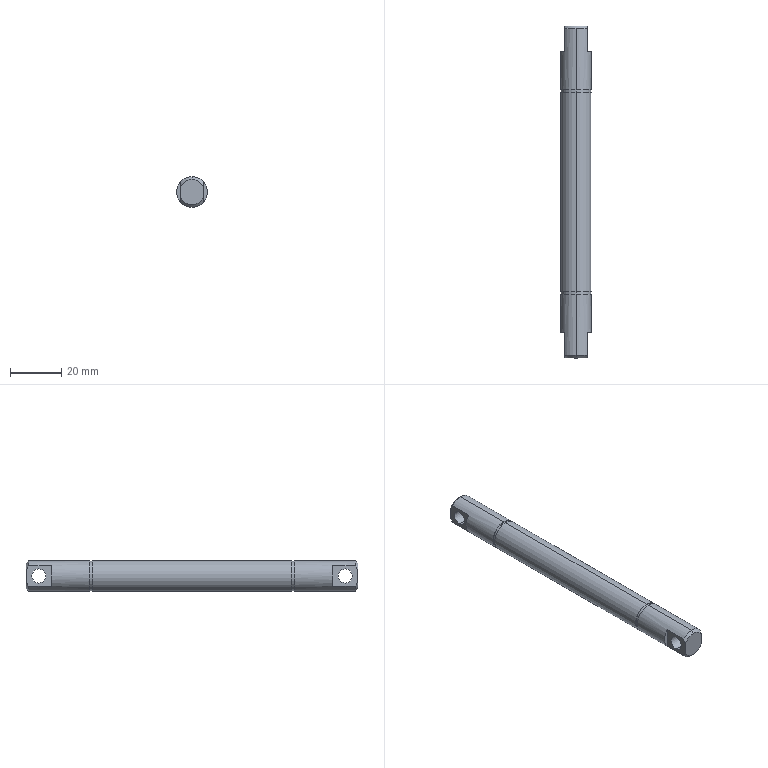Part | SolidWorks | features ICE 3, MirrorPattern 3, Chamfer 1, Extrusion 1 | 1 solid | 34 faces | box 12 x 130 x 12 mm | volume 13909 mm3 | cylinder 14 | plane 14 | cone 6 | commonest cylinder face diameters 12 x6 5.5 x4 11.5 x4
STEP:
#1=CARTESIAN_POINT('',(0.,25.,6.));
#2=VERTEX_POINT('',#1);
#3=CARTESIAN_POINT('',(0.,25.,-6.));
#4=VERTEX_POINT('',#3);
#5=CARTESIAN_POINT('',(0.,25.,0.));
#6=DIRECTION('',(0.,1.,0.));
#7=DIRECTION('',(0.,0.,1.));
#8=AXIS2_PLACEMENT_3D('',#5,#6,#7);
#9=CIRCLE('',#8,6.);
#10=EDGE_CURVE('',#2,#4,#9,.T.);
#11=ORIENTED_EDGE('',*,*,#10,.F.);
#12=CARTESIAN_POINT('',(0.,1.,6.));
#13=VERTEX_POINT('',#12);
#14=CARTESIAN_POINT('',(0.,130.,6.));
#15=DIRECTION('',(0.,-1.,0.));
#16=VECTOR('',#15,1000.);
#17=LINE('',#14,#16);
#18=EDGE_CURVE('',#2,#13,#17,.T.);
#19=ORIENTED_EDGE('',*,*,#18,.T.);
#20=CARTESIAN_POINT('',(4.5,1.,3.969));
#21=VERTEX_POINT('',#20);
#22=CARTESIAN_POINT('',(0.,1.,0.));
#23=DIRECTION('',(0.,1.,0.));
#24=DIRECTION('',(0.,0.,1.));
#25=AXIS2_PLACEMENT_3D('',#22,#23,#24);
#26=CIRCLE('',#25,6.);
#27=EDGE_CURVE('',#13,#21,#26,.T.);
#28=ORIENTED_EDGE('',*,*,#27,.T.);
#29=CARTESIAN_POINT('',(4.5,10.,3.969));
#30=VERTEX_POINT('',#29);
#31=CARTESIAN_POINT('',(4.5,130.,3.969));
#32=DIRECTION('',(0.,1.,0.));
#33=VECTOR('',#32,1000.);
#34=LINE('',#31,#33);
#35=EDGE_CURVE('',#21,#30,#34,.T.);
#36=ORIENTED_EDGE('',*,*,#35,.T.);
#37=CARTESIAN_POINT('',(4.5,10.,-3.969));
#38=VERTEX_POINT('',#37);
#39=CARTESIAN_POINT('',(0.,10.,0.));
#40=DIRECTION('',(0.,1.,0.));
#41=DIRECTION('',(0.,0.,1.));
#42=AXIS2_PLACEMENT_3D('',#39,#40,#41);
#43=CIRCLE('',#42,6.);
#44=EDGE_CURVE('',#30,#38,#43,.T.);
#45=ORIENTED_EDGE('',*,*,#44,.T.);
#46=CARTESIAN_POINT('',(4.5,1.,-3.969));
#47=VERTEX_POINT('',#46);
#48=CARTESIAN_POINT('',(4.5,130.,-3.969));
#49=DIRECTION('',(0.,-1.,0.));
#50=VECTOR('',#49,1000.);
#51=LINE('',#48,#50);
#52=EDGE_CURVE('',#38,#47,#51,.T.);
#53=ORIENTED_EDGE('',*,*,#52,.T.);
#54=CARTESIAN_POINT('',(0.,1.,-6.));
#55=VERTEX_POINT('',#54);
#56=CARTESIAN_POINT('',(0.,1.,0.));
#57=DIRECTION('',(0.,1.,0.));
#58=DIRECTION('',(0.,0.,1.));
#59=AXIS2_PLACEMENT_3D('',#56,#57,#58);
#60=CIRCLE('',#59,6.);
#61=EDGE_CURVE('',#47,#55,#60,.T.);
#62=ORIENTED_EDGE('',*,*,#61,.T.);
#63=CARTESIAN_POINT('',(0.,130.,-6.));
#64=DIRECTION('',(0.,-1.,0.));
#65=VECTOR('',#64,1000.);
#66=LINE('',#63,#65);
#67=EDGE_CURVE('',#4,#55,#66,.T.);
#68=ORIENTED_EDGE('',*,*,#67,.F.);
#69=EDGE_LOOP('',(#11,#19,#28,#36,#45,#53,#62,#68));
#70=FACE_OUTER_BOUND('',#69,.T.);
#71=CARTESIAN_POINT('',(0.,130.,0.));
#72=DIRECTION('',(0.,-1.,0.));
#73=DIRECTION('',(0.,0.,-1.));
#74=AXIS2_PLACEMENT_3D('',#71,#72,#73);
#75=CYLINDRICAL_SURFACE('',#74,6.);
#76=ADVANCED_FACE('',(#70),#75,.T.);
#77=CARTESIAN_POINT('',(0.,0.,5.));
#78=VERTEX_POINT('',#77);
#79=CARTESIAN_POINT('',(-4.5,0.,2.179));
#80=VERTEX_POINT('',#79);
#81=CARTESIAN_POINT('',(0.,0.,0.));
#82=DIRECTION('',(0.,-1.,0.));
#83=DIRECTION('',(0.,0.,1.));
#84=AXIS2_PLACEMENT_3D('',#81,#82,#83);
#85=CIRCLE('',#84,5.);
#86=EDGE_CURVE('',#78,#80,#85,.T.);
#87=ORIENTED_EDGE('',*,*,#86,.F.);
#88=CARTESIAN_POINT('',(0.,1.,6.));
#89=DIRECTION('',(0.,0.7071,0.7071));
#90=VECTOR('',#89,1000.);
#91=LINE('',#88,#90);
#92=EDGE_CURVE('',#78,#13,#91,.T.);
#93=ORIENTED_EDGE('',*,*,#92,.T.);
#94=CARTESIAN_POINT('',(-4.5,1.,3.969));
#95=VERTEX_POINT('',#94);
#96=CARTESIAN_POINT('',(0.,1.,0.));
#97=DIRECTION('',(0.,1.,0.));
#98=DIRECTION('',(0.,0.,1.));
#99=AXIS2_PLACEMENT_3D('',#96,#97,#98);
#100=CIRCLE('',#99,6.);
#101=EDGE_CURVE('',#95,#13,#100,.T.);
#102=ORIENTED_EDGE('',*,*,#101,.F.);
#103=CARTESIAN_POINT('',(-4.5,0.,2.179));
#104=CARTESIAN_POINT('',(-4.5,0.2738,2.808));
#105=CARTESIAN_POINT('',(-4.5,0.6215,3.396));
#106=CARTESIAN_POINT('',(-4.5,1.,3.969));
#107=B_SPLINE_CURVE_WITH_KNOTS('',3,(#103,#104,#105,#106),.UNSPECIFIED.,.F.,.F.,(4,4),(0.006523,0.008562),.UNSPECIFIED.);
#108=EDGE_CURVE('',#80,#95,#107,.T.);
#109=ORIENTED_EDGE('',*,*,#108,.F.);
#110=EDGE_LOOP('',(#87,#93,#102,#109));
#111=FACE_OUTER_BOUND('',#110,.T.);
#112=CARTESIAN_POINT('',(0.,1.,0.));
#113=DIRECTION('',(0.,1.,0.));
#114=DIRECTION('',(0.,0.,1.));
#115=AXIS2_PLACEMENT_3D('',#112,#113,#114);
#116=CONICAL_SURFACE('',#115,6.,0.7854);
#117=ADVANCED_FACE('',(#111),#116,.T.);
#118=CARTESIAN_POINT('',(-4.5,5.,-2.75));
#119=VERTEX_POINT('',#118);
#120=CARTESIAN_POINT('',(-4.5,5.,2.75));
#121=VERTEX_POINT('',#120);
#122=CARTESIAN_POINT('',(-4.5,5.,0.));
#123=DIRECTION('',(-1.,0.,0.));
#124=DIRECTION('',(0.,0.,-1.));
#125=AXIS2_PLACEMENT_3D('',#122,#123,#124);
#126=CIRCLE('',#125,2.75);
#127=EDGE_CURVE('',#119,#121,#126,.T.);
#128=ORIENTED_EDGE('',*,*,#127,.T.);
#129=CARTESIAN_POINT('',(4.5,5.,2.75));
#130=VERTEX_POINT('',#129);
#131=CARTESIAN_POINT('',(-6.,5.,2.75));
#132=DIRECTION('',(1.,0.,0.));
#133=VECTOR('',#132,1000.);
#134=LINE('',#131,#133);
#135=EDGE_CURVE('',#121,#130,#134,.T.);
#136=ORIENTED_EDGE('',*,*,#135,.T.);
#137=CARTESIAN_POINT('',(4.5,5.,-2.75));
#138=VERTEX_POINT('',#137);
#139=CARTESIAN_POINT('',(4.5,5.,0.));
#140=DIRECTION('',(1.,0.,0.));
#141=DIRECTION('',(0.,0.,1.));
#142=AXIS2_PLACEMENT_3D('',#139,#140,#141);
#143=CIRCLE('',#142,2.75);
#144=EDGE_CURVE('',#130,#138,#143,.T.);
#145=ORIENTED_EDGE('',*,*,#144,.T.);
#146=CARTESIAN_POINT('',(-6.,5.,-2.75));
#147=DIRECTION('',(1.,0.,0.));
#148=VECTOR('',#147,1000.);
#149=LINE('',#146,#148);
#150=EDGE_CURVE('',#119,#138,#149,.T.);
#151=ORIENTED_EDGE('',*,*,#150,.F.);
#152=EDGE_LOOP('',(#128,#136,#145,#151));
#153=FACE_OUTER_BOUND('',#152,.T.);
#154=CARTESIAN_POINT('',(-6.,5.,0.));
#155=DIRECTION('',(1.,0.,0.));
#156=DIRECTION('',(0.,0.,-1.));
#157=AXIS2_PLACEMENT_3D('',#154,#155,#156);
#158=CYLINDRICAL_SURFACE('',#157,2.75);
#159=ADVANCED_FACE('',(#153),#158,.F.);
#160=CARTESIAN_POINT('',(0.,25.,5.75));
#161=VERTEX_POINT('',#160);
#162=CARTESIAN_POINT('',(0.,25.,-5.75));
#163=VERTEX_POINT('',#162);
#164=CARTESIAN_POINT('',(0.,25.,0.));
#165=DIRECTION('',(0.,1.,0.));
#166=DIRECTION('',(0.,0.,1.));
#167=AXIS2_PLACEMENT_3D('',#164,#165,#166);
#168=CIRCLE('',#167,5.75);
#169=EDGE_CURVE('',#161,#163,#168,.T.);
#170=ORIENTED_EDGE('',*,*,#169,.T.);
#171=CARTESIAN_POINT('',(0.,26.,-5.75));
#172=VERTEX_POINT('',#171);
#173=CARTESIAN_POINT('',(0.,25.,-5.75));
#174=DIRECTION('',(0.,1.,0.));
#175=VECTOR('',#174,1000.);
#176=LINE('',#173,#175);
#177=EDGE_CURVE('',#163,#172,#176,.T.);
#178=ORIENTED_EDGE('',*,*,#177,.T.);
#179=CARTESIAN_POINT('',(0.,26.,5.75));
#180=VERTEX_POINT('',#179);
#181=CARTESIAN_POINT('',(0.,26.,0.));
#182=DIRECTION('',(0.,1.,0.));
#183=DIRECTION('',(0.,0.,1.));
#184=AXIS2_PLACEMENT_3D('',#181,#182,#183);
#185=CIRCLE('',#184,5.75);
#186=EDGE_CURVE('',#180,#172,#185,.T.);
#187=ORIENTED_EDGE('',*,*,#186,.F.);
#188=CARTESIAN_POINT('',(0.,25.,5.75));
#189=DIRECTION('',(0.,1.,0.));
#190=VECTOR('',#189,1000.);
#191=LINE('',#188,#190);
#192=EDGE_CURVE('',#161,#180,#191,.T.);
#193=ORIENTED_EDGE('',*,*,#192,.F.);
#194=EDGE_LOOP('',(#170,#178,#187,#193));
#195=FACE_OUTER_BOUND('',#194,.T.);
#196=CARTESIAN_POINT('',(0.,25.,0.));
#197=DIRECTION('',(0.,1.,0.));
#198=DIRECTION('',(0.,0.,1.));
#199=AXIS2_PLACEMENT_3D('',#196,#197,#198);
#200=CYLINDRICAL_SURFACE('',#199,5.75);
#201=ADVANCED_FACE('',(#195),#200,.T.);
#202=CARTESIAN_POINT('',(0.,105.,5.75));
#203=VERTEX_POINT('',#202);
#204=CARTESIAN_POINT('',(0.,105.,-5.75));
#205=VERTEX_POINT('',#204);
#206=CARTESIAN_POINT('',(0.,105.,0.));
#207=DIRECTION('',(0.,1.,0.));
#208=DIRECTION('',(0.,0.,1.));
#209=AXIS2_PLACEMENT_3D('',#206,#207,#208);
#210=CIRCLE('',#209,5.75);
#211=EDGE_CURVE('',#203,#205,#210,.T.);
#212=ORIENTED_EDGE('',*,*,#211,.F.);
#213=CARTESIAN_POINT('',(0.,104.,5.75));
#214=VERTEX_POINT('',#213);
#215=CARTESIAN_POINT('',(0.,105.,5.75));
#216=DIRECTION('',(0.,-1.,0.));
#217=VECTOR('',#216,1000.);
#218=LINE('',#215,#217);
#219=EDGE_CURVE('',#203,#214,#218,.T.);
#220=ORIENTED_EDGE('',*,*,#219,.T.);
#221=CARTESIAN_POINT('',(0.,104.,-5.75));
#222=VERTEX_POINT('',#221);
#223=CARTESIAN_POINT('',(0.,104.,0.));
#224=DIRECTION('',(0.,1.,0.));
#225=DIRECTION('',(0.,0.,1.));
#226=AXIS2_PLACEMENT_3D('',#223,#224,#225);
#227=CIRCLE('',#226,5.75);
#228=EDGE_CURVE('',#214,#222,#227,.T.);
#229=ORIENTED_EDGE('',*,*,#228,.T.);
#230=CARTESIAN_POINT('',(0.,105.,-5.75));
#231=DIRECTION('',(0.,-1.,0.));
#232=VECTOR('',#231,1000.);
#233=LINE('',#230,#232);
#234=EDGE_CURVE('',#205,#222,#233,.T.);
#235=ORIENTED_EDGE('',*,*,#234,.F.);
#236=EDGE_LOOP('',(#212,#220,#229,#235));
#237=FACE_OUTER_BOUND('',#236,.T.);
#238=CARTESIAN_POINT('',(0.,105.,0.));
#239=DIRECTION('',(0.,-1.,0.));
#240=DIRECTION('',(0.,0.,-1.));
#241=AXIS2_PLACEMENT_3D('',#238,#239,#240);
#242=CYLINDRICAL_SURFACE('',#241,5.75);
#243=ADVANCED_FACE('',(#237),#242,.T.);
#244=CARTESIAN_POINT('',(-4.5,125.,-2.75));
#245=VERTEX_POINT('',#244);
#246=CARTESIAN_POINT('',(-4.5,125.,2.75));
#247=VERTEX_POINT('',#246);
#248=CARTESIAN_POINT('',(-4.5,125.,0.));
#249=DIRECTION('',(-1.,0.,0.));
#250=DIRECTION('',(0.,0.,-1.));
#251=AXIS2_PLACEMENT_3D('',#248,#249,#250);
#252=CIRCLE('',#251,2.75);
#253=EDGE_CURVE('',#245,#247,#252,.T.);
#254=ORIENTED_EDGE('',*,*,#253,.T.);
#255=CARTESIAN_POINT('',(4.5,125.,2.75));
#256=VERTEX_POINT('',#255);
#257=CARTESIAN_POINT('',(-6.,125.,2.75));
#258=DIRECTION('',(1.,0.,0.));
#259=VECTOR('',#258,1000.);
#260=LINE('',#257,#259);
#261=EDGE_CURVE('',#247,#256,#260,.T.);
#262=ORIENTED_EDGE('',*,*,#261,.T.);
#263=CARTESIAN_POINT('',(4.5,125.,-2.75));
#264=VERTEX_POINT('',#263);
#265=CARTESIAN_POINT('',(4.5,125.,0.));
#266=DIRECTION('',(1.,0.,0.));
#267=DIRECTION('',(0.,0.,1.));
#268=AXIS2_PLACEMENT_3D('',#265,#266,#267);
#269=CIRCLE('',#268,2.75);
#270=EDGE_CURVE('',#256,#264,#269,.T.);
#271=ORIENTED_EDGE('',*,*,#270,.T.);
#272=CARTESIAN_POINT('',(-6.,125.,-2.75));
#273=DIRECTION('',(1.,0.,0.));
#274=VECTOR('',#273,1000.);
#275=LINE('',#272,#274);
#276=EDGE_CURVE('',#245,#264,#275,.T.);
#277=ORIENTED_EDGE('',*,*,#276,.F.);
#278=EDGE_LOOP('',(#254,#262,#271,#277));
#279=FACE_OUTER_BOUND('',#278,.T.);
#280=CARTESIAN_POINT('',(-6.,125.,0.));
#281=DIRECTION('',(1.,0.,0.));
#282=DIRECTION('',(0.,0.,-1.));
#283=AXIS2_PLACEMENT_3D('',#280,#281,#282);
#284=CYLINDRICAL_SURFACE('',#283,2.75);
#285=ADVANCED_FACE('',(#279),#284,.F.);
#286=CARTESIAN_POINT('',(0.,130.,-5.));
#287=VERTEX_POINT('',#286);
#288=CARTESIAN_POINT('',(-4.5,130.,-2.179));
#289=VERTEX_POINT('',#288);
#290=CARTESIAN_POINT('',(0.,130.,0.));
#291=DIRECTION('',(0.,1.,0.));
#292=DIRECTION('',(0.,0.,1.));
#293=AXIS2_PLACEMENT_3D('',#290,#291,#292);
#294=CIRCLE('',#293,5.);
#295=EDGE_CURVE('',#287,#289,#294,.T.);
#296=ORIENTED_EDGE('',*,*,#295,.F.);
#297=CARTESIAN_POINT('',(0.,129.,-6.));
#298=VERTEX_POINT('',#297);
#299=CARTESIAN_POINT('',(0.,130.,-5.));
#300=DIRECTION('',(0.,-0.7071,-0.7071));
#301=VECTOR('',#300,1000.);
#302=LINE('',#299,#301);
#303=EDGE_CURVE('',#287,#298,#302,.T.);
#304=ORIENTED_EDGE('',*,*,#303,.T.);
#305=CARTESIAN_POINT('',(-4.5,129.,-3.969));
#306=VERTEX_POINT('',#305);
#307=CARTESIAN_POINT('',(0.,129.,0.));
#308=DIRECTION('',(0.,-1.,0.));
#309=DIRECTION('',(0.,0.,1.));
#310=AXIS2_PLACEMENT_3D('',#307,#308,#309);
#311=CIRCLE('',#310,6.);
#312=EDGE_CURVE('',#306,#298,#311,.T.);
#313=ORIENTED_EDGE('',*,*,#312,.F.);
#314=CARTESIAN_POINT('',(-4.5,130.,-2.179));
#315=CARTESIAN_POINT('',(-4.5,129.726,-2.808));
#316=CARTESIAN_POINT('',(-4.5,129.379,-3.396));
#317=CARTESIAN_POINT('',(-4.5,129.,-3.969));
#318=B_SPLINE_CURVE_WITH_KNOTS('',3,(#314,#315,#316,#317),.UNSPECIFIED.,.F.,.F.,(4,4),(0.006523,0.008562),.UNSPECIFIED.);
#319=EDGE_CURVE('',#289,#306,#318,.T.);
#320=ORIENTED_EDGE('',*,*,#319,.F.);
#321=EDGE_LOOP('',(#296,#304,#313,#320));
#322=FACE_OUTER_BOUND('',#321,.T.);
#323=CARTESIAN_POINT('',(0.,130.,0.));
#324=DIRECTION('',(0.,-1.,0.));
#325=DIRECTION('',(0.,0.,-1.));
#326=AXIS2_PLACEMENT_3D('',#323,#324,#325);
#327=CONICAL_SURFACE('',#326,5.,0.7854);
#328=ADVANCED_FACE('',(#322),#327,.T.);
#329=CARTESIAN_POINT('',(4.5,129.,3.969));
#330=VERTEX_POINT('',#329);
#331=CARTESIAN_POINT('',(0.,129.,6.));
#332=VERTEX_POINT('',#331);
#333=CARTESIAN_POINT('',(0.,129.,0.));
#334=DIRECTION('',(0.,-1.,0.));
#335=DIRECTION('',(0.,0.,1.));
#336=AXIS2_PLACEMENT_3D('',#333,#334,#335);
#337=CIRCLE('',#336,6.);
#338=EDGE_CURVE('',#330,#332,#337,.T.);
#339=ORIENTED_EDGE('',*,*,#338,.T.);
#340=CARTESIAN_POINT('',(0.,105.,6.));
#341=VERTEX_POINT('',#340);
#342=CARTESIAN_POINT('',(0.,130.,6.));
#343=DIRECTION('',(0.,-1.,0.));
#344=VECTOR('',#343,1000.);
#345=LINE('',#342,#344);
#346=EDGE_CURVE('',#332,#341,#345,.T.);
#347=ORIENTED_EDGE('',*,*,#346,.T.);
#348=CARTESIAN_POINT('',(0.,105.,-6.));
#349=VERTEX_POINT('',#348);
#350=CARTESIAN_POINT('',(0.,105.,0.));
#351=DIRECTION('',(0.,1.,0.));
#352=DIRECTION('',(0.,0.,1.));
#353=AXIS2_PLACEMENT_3D('',#350,#351,#352);
#354=CIRCLE('',#353,6.);
#355=EDGE_CURVE('',#341,#349,#354,.T.);
#356=ORIENTED_EDGE('',*,*,#355,.T.);
#357=CARTESIAN_POINT('',(0.,130.,-6.));
#358=DIRECTION('',(0.,-1.,0.));
#359=VECTOR('',#358,1000.);
#360=LINE('',#357,#359);
#361=EDGE_CURVE('',#298,#349,#360,.T.);
#362=ORIENTED_EDGE('',*,*,#361,.F.);
#363=CARTESIAN_POINT('',(4.5,129.,-3.969));
#364=VERTEX_POINT('',#363);
#365=CARTESIAN_POINT('',(0.,129.,0.));
#366=DIRECTION('',(0.,-1.,0.));
#367=DIRECTION('',(0.,0.,1.));
#368=AXIS2_PLACEMENT_3D('',#365,#366,#367);
#369=CIRCLE('',#368,6.);
#370=EDGE_CURVE('',#298,#364,#369,.T.);
#371=ORIENTED_EDGE('',*,*,#370,.T.);
#372=CARTESIAN_POINT('',(4.5,120.,-3.969));
#373=VERTEX_POINT('',#372);
#374=CARTESIAN_POINT('',(4.5,130.,-3.969));
#375=DIRECTION('',(0.,-1.,0.));
#376=VECTOR('',#375,1000.);
#377=LINE('',#374,#376);
#378=EDGE_CURVE('',#364,#373,#377,.T.);
#379=ORIENTED_EDGE('',*,*,#378,.T.);
#380=CARTESIAN_POINT('',(4.5,120.,3.969));
#381=VERTEX_POINT('',#380);
#382=CARTESIAN_POINT('',(0.,120.,0.));
#383=DIRECTION('',(0.,1.,0.));
#384=DIRECTION('',(0.,0.,1.));
#385=AXIS2_PLACEMENT_3D('',#382,#383,#384);
#386=CIRCLE('',#385,6.);
#387=EDGE_CURVE('',#381,#373,#386,.T.);
#388=ORIENTED_EDGE('',*,*,#387,.F.);
#389=CARTESIAN_POINT('',(4.5,130.,3.969));
#390=DIRECTION('',(0.,1.,0.));
#391=VECTOR('',#390,1000.);
#392=LINE('',#389,#391);
#393=EDGE_CURVE('',#381,#330,#392,.T.);
#394=ORIENTED_EDGE('',*,*,#393,.T.);
#395=EDGE_LOOP('',(#339,#347,#356,#362,#371,#379,#388,#394));
#396=FACE_OUTER_BOUND('',#395,.T.);
#397=CARTESIAN_POINT('',(0.,130.,0.));
#398=DIRECTION('',(0.,-1.,0.));
#399=DIRECTION('',(0.,0.,-1.));
#400=AXIS2_PLACEMENT_3D('',#397,#398,#399);
#401=CYLINDRICAL_SURFACE('',#400,6.);
#402=ADVANCED_FACE('',(#396),#401,.T.);
#403=CARTESIAN_POINT('',(0.,104.,6.));
#404=VERTEX_POINT('',#403);
#405=CARTESIAN_POINT('',(0.,104.,-6.));
#406=VERTEX_POINT('',#405);
#407=CARTESIAN_POINT('',(0.,104.,0.));
#408=DIRECTION('',(0.,1.,0.));
#409=DIRECTION('',(0.,0.,1.));
#410=AXIS2_PLACEMENT_3D('',#407,#408,#409);
#411=CIRCLE('',#410,6.);
#412=EDGE_CURVE('',#404,#406,#411,.T.);
#413=ORIENTED_EDGE('',*,*,#412,.F.);
#414=CARTESIAN_POINT('',(0.,26.,6.));
#415=VERTEX_POINT('',#414);
#416=CARTESIAN_POINT('',(0.,130.,6.));
#417=DIRECTION('',(0.,-1.,0.));
#418=VECTOR('',#417,1000.);
#419=LINE('',#416,#418);
#420=EDGE_CURVE('',#404,#415,#419,.T.);
#421=ORIENTED_EDGE('',*,*,#420,.T.);
#422=CARTESIAN_POINT('',(0.,26.,-6.));
#423=VERTEX_POINT('',#422);
#424=CARTESIAN_POINT('',(0.,26.,0.));
#425=DIRECTION('',(0.,1.,0.));
#426=DIRECTION('',(0.,0.,1.));
#427=AXIS2_PLACEMENT_3D('',#424,#425,#426);
#428=CIRCLE('',#427,6.);
#429=EDGE_CURVE('',#415,#423,#428,.T.);
#430=ORIENTED_EDGE('',*,*,#429,.T.);
#431=CARTESIAN_POINT('',(0.,130.,-6.));
#432=DIRECTION('',(0.,-1.,0.));
#433=VECTOR('',#432,1000.);
#434=LINE('',#431,#433);
#435=EDGE_CURVE('',#406,#423,#434,.T.);
#436=ORIENTED_EDGE('',*,*,#435,.F.);
#437=EDGE_LOOP('',(#413,#421,#430,#436));
#438=FACE_OUTER_BOUND('',#437,.T.);
#439=CARTESIAN_POINT('',(0.,130.,0.));
#440=DIRECTION('',(0.,-1.,0.));
#441=DIRECTION('',(0.,0.,-1.));
#442=AXIS2_PLACEMENT_3D('',#439,#440,#441);
#443=CYLINDRICAL_SURFACE('',#442,6.);
#444=ADVANCED_FACE('',(#438),#443,.T.);
#445=ORIENTED_EDGE('',*,*,#420,.F.);
#446=CARTESIAN_POINT('',(0.,104.,0.));
#447=DIRECTION('',(0.,1.,0.));
#448=DIRECTION('',(0.,0.,1.));
#449=AXIS2_PLACEMENT_3D('',#446,#447,#448);
#450=CIRCLE('',#449,6.);
#451=EDGE_CURVE('',#406,#404,#450,.T.);
#452=ORIENTED_EDGE('',*,*,#451,.F.);
#453=ORIENTED_EDGE('',*,*,#435,.T.);
#454=CARTESIAN_POINT('',(0.,26.,0.));
#455=DIRECTION('',(0.,1.,0.));
#456=DIRECTION('',(0.,0.,1.));
#457=AXIS2_PLACEMENT_3D('',#454,#455,#456);
#458=CIRCLE('',#457,6.);
#459=EDGE_CURVE('',#423,#415,#458,.T.);
#460=ORIENTED_EDGE('',*,*,#459,.T.);
#461=EDGE_LOOP('',(#445,#452,#453,#460));
#462=FACE_OUTER_BOUND('',#461,.T.);
#463=CARTESIAN_POINT('',(0.,130.,0.));
#464=DIRECTION('',(0.,-1.,0.));
#465=DIRECTION('',(0.,0.,-1.));
#466=AXIS2_PLACEMENT_3D('',#463,#464,#465);
#467=CYLINDRICAL_SURFACE('',#466,6.);
#468=ADVANCED_FACE('',(#462),#467,.T.);
#469=ORIENTED_EDGE('',*,*,#346,.F.);
#470=CARTESIAN_POINT('',(-4.5,129.,3.969));
#471=VERTEX_POINT('',#470);
#472=CARTESIAN_POINT('',(0.,129.,0.));
#473=DIRECTION('',(0.,-1.,0.));
#474=DIRECTION('',(0.,0.,1.));
#475=AXIS2_PLACEMENT_3D('',#472,#473,#474);
#476=CIRCLE('',#475,6.);
#477=EDGE_CURVE('',#332,#471,#476,.T.);
#478=ORIENTED_EDGE('',*,*,#477,.T.);
#479=CARTESIAN_POINT('',(-4.5,120.,3.969));
#480=VERTEX_POINT('',#479);
#481=CARTESIAN_POINT('',(-4.5,130.,3.969));
#482=DIRECTION('',(0.,-1.,0.));
#483=VECTOR('',#482,1000.);
#484=LINE('',#481,#483);
#485=EDGE_CURVE('',#471,#480,#484,.T.);
#486=ORIENTED_EDGE('',*,*,#485,.T.);
#487=CARTESIAN_POINT('',(-4.5,120.,-3.969));
#488=VERTEX_POINT('',#487);
#489=CARTESIAN_POINT('',(0.,120.,0.));
#490=DIRECTION('',(0.,-1.,0.));
#491=DIRECTION('',(0.,0.,-1.));
#492=AXIS2_PLACEMENT_3D('',#489,#490,#491);
#493=CIRCLE('',#492,6.);
#494=EDGE_CURVE('',#480,#488,#493,.T.);
#495=ORIENTED_EDGE('',*,*,#494,.T.);
#496=CARTESIAN_POINT('',(-4.5,130.,-3.969));
#497=DIRECTION('',(0.,1.,0.));
#498=VECTOR('',#497,1000.);
#499=LINE('',#496,#498);
#500=EDGE_CURVE('',#488,#306,#499,.T.);
#501=ORIENTED_EDGE('',*,*,#500,.T.);
#502=ORIENTED_EDGE('',*,*,#312,.T.);
#503=ORIENTED_EDGE('',*,*,#361,.T.);
#504=CARTESIAN_POINT('',(0.,105.,0.));
#505=DIRECTION('',(0.,1.,0.));
#506=DIRECTION('',(0.,0.,1.));
#507=AXIS2_PLACEMENT_3D('',#504,#505,#506);
#508=CIRCLE('',#507,6.);
#509=EDGE_CURVE('',#349,#341,#508,.T.);
#510=ORIENTED_EDGE('',*,*,#509,.T.);
#511=EDGE_LOOP('',(#469,#478,#486,#495,#501,#502,#503,#510));
#512=FACE_OUTER_BOUND('',#511,.T.);
#513=CARTESIAN_POINT('',(0.,130.,0.));
#514=DIRECTION('',(0.,-1.,0.));
#515=DIRECTION('',(0.,0.,-1.));
#516=AXIS2_PLACEMENT_3D('',#513,#514,#515);
#517=CYLINDRICAL_SURFACE('',#516,6.);
#518=ADVANCED_FACE('',(#512),#517,.T.);
#519=ORIENTED_EDGE('',*,*,#303,.F.);
#520=CARTESIAN_POINT('',(4.5,130.,-2.179));
#521=VERTEX_POINT('',#520);
#522=CARTESIAN_POINT('',(0.,130.,0.));
#523=DIRECTION('',(0.,1.,0.));
#524=DIRECTION('',(0.,0.,1.));
#525=AXIS2_PLACEMENT_3D('',#522,#523,#524);
#526=CIRCLE('',#525,5.);
#527=EDGE_CURVE('',#521,#287,#526,.T.);
#528=ORIENTED_EDGE('',*,*,#527,.F.);
#529=CARTESIAN_POINT('',(4.5,129.,-3.969));
#530=CARTESIAN_POINT('',(4.5,129.379,-3.395));
#531=CARTESIAN_POINT('',(4.5,129.727,-2.806));
#532=CARTESIAN_POINT('',(4.5,130.,-2.179));
#533=B_SPLINE_CURVE_WITH_KNOTS('',3,(#529,#530,#531,#532),.UNSPECIFIED.,.F.,.F.,(4,4),(0.00000126,0.002049),.UNSPECIFIED.);
#534=EDGE_CURVE('',#364,#521,#533,.T.);
#535=ORIENTED_EDGE('',*,*,#534,.F.);
#536=ORIENTED_EDGE('',*,*,#370,.F.);
#537=EDGE_LOOP('',(#519,#528,#535,#536));
#538=FACE_OUTER_BOUND('',#537,.T.);
#539=CARTESIAN_POINT('',(0.,130.,0.));
#540=DIRECTION('',(0.,-1.,0.));
#541=DIRECTION('',(0.,0.,-1.));
#542=AXIS2_PLACEMENT_3D('',#539,#540,#541);
#543=CONICAL_SURFACE('',#542,5.,0.7854);
#544=ADVANCED_FACE('',(#538),#543,.T.);
#545=CARTESIAN_POINT('',(4.5,130.,2.179));
#546=VERTEX_POINT('',#545);
#547=CARTESIAN_POINT('',(4.5,130.,0.));
#548=DIRECTION('',(0.,0.,1.));
#549=VECTOR('',#548,1000.);
#550=LINE('',#547,#549);
#551=EDGE_CURVE('',#521,#546,#550,.T.);
#552=ORIENTED_EDGE('',*,*,#551,.F.);
#553=ORIENTED_EDGE('',*,*,#527,.T.);
#554=ORIENTED_EDGE('',*,*,#295,.T.);
#555=CARTESIAN_POINT('',(-4.5,130.,2.179));
#556=VERTEX_POINT('',#555);
#557=CARTESIAN_POINT('',(-4.5,130.,0.));
#558=DIRECTION('',(0.,0.,-1.));
#559=VECTOR('',#558,1000.);
#560=LINE('',#557,#559);
#561=EDGE_CURVE('',#556,#289,#560,.T.);
#562=ORIENTED_EDGE('',*,*,#561,.F.);
#563=CARTESIAN_POINT('',(0.,130.,0.));
#564=DIRECTION('',(0.,1.,0.));
#565=DIRECTION('',(0.,0.,1.));
#566=AXIS2_PLACEMENT_3D('',#563,#564,#565);
#567=CIRCLE('',#566,5.);
#568=EDGE_CURVE('',#556,#546,#567,.T.);
#569=ORIENTED_EDGE('',*,*,#568,.T.);
#570=EDGE_LOOP('',(#552,#553,#554,#562,#569));
#571=FACE_OUTER_BOUND('',#570,.T.);
#572=CARTESIAN_POINT('',(0.,130.,0.));
#573=DIRECTION('',(0.,1.,0.));
#574=DIRECTION('',(0.,0.,1.));
#575=AXIS2_PLACEMENT_3D('',#572,#573,#574);
#576=PLANE('',#575);
#577=ADVANCED_FACE('',(#571),#576,.T.);
#578=ORIENTED_EDGE('',*,*,#261,.F.);
#579=CARTESIAN_POINT('',(-4.5,125.,0.));
#580=DIRECTION('',(-1.,0.,0.));
#581=DIRECTION('',(0.,0.,-1.));
#582=AXIS2_PLACEMENT_3D('',#579,#580,#581);
#583=CIRCLE('',#582,2.75);
#584=EDGE_CURVE('',#247,#245,#583,.T.);
#585=ORIENTED_EDGE('',*,*,#584,.T.);
#586=ORIENTED_EDGE('',*,*,#276,.T.);
#587=CARTESIAN_POINT('',(4.5,125.,0.));
#588=DIRECTION('',(1.,0.,0.));
#589=DIRECTION('',(0.,0.,1.));
#590=AXIS2_PLACEMENT_3D('',#587,#588,#589);
#591=CIRCLE('',#590,2.75);
#592=EDGE_CURVE('',#264,#256,#591,.T.);
#593=ORIENTED_EDGE('',*,*,#592,.T.);
#594=EDGE_LOOP('',(#578,#585,#586,#593));
#595=FACE_OUTER_BOUND('',#594,.T.);
#596=CARTESIAN_POINT('',(-6.,125.,0.));
#597=DIRECTION('',(1.,0.,0.));
#598=DIRECTION('',(0.,0.,-1.));
#599=AXIS2_PLACEMENT_3D('',#596,#597,#598);
#600=CYLINDRICAL_SURFACE('',#599,2.75);
#601=ADVANCED_FACE('',(#595),#600,.F.);
#602=CARTESIAN_POINT('',(4.5,130.,2.179));
#603=CARTESIAN_POINT('',(4.5,129.726,2.808));
#604=CARTESIAN_POINT('',(4.5,129.379,3.396));
#605=CARTESIAN_POINT('',(4.5,129.,3.969));
#606=B_SPLINE_CURVE_WITH_KNOTS('',3,(#602,#603,#604,#605),.UNSPECIFIED.,.F.,.F.,(4,4),(0.006523,0.008562),.UNSPECIFIED.);
#607=EDGE_CURVE('',#546,#330,#606,.T.);
#608=ORIENTED_EDGE('',*,*,#607,.F.);
#609=ORIENTED_EDGE('',*,*,#568,.F.);
#610=CARTESIAN_POINT('',(-4.5,129.,3.969));
#611=CARTESIAN_POINT('',(-4.5,129.379,3.395));
#612=CARTESIAN_POINT('',(-4.5,129.727,2.806));
#613=CARTESIAN_POINT('',(-4.5,130.,2.179));
#614=B_SPLINE_CURVE_WITH_KNOTS('',3,(#610,#611,#612,#613),.UNSPECIFIED.,.F.,.F.,(4,4),(0.00000126,0.002049),.UNSPECIFIED.);
#615=EDGE_CURVE('',#471,#556,#614,.T.);
#616=ORIENTED_EDGE('',*,*,#615,.F.);
#617=ORIENTED_EDGE('',*,*,#477,.F.);
#618=ORIENTED_EDGE('',*,*,#338,.F.);
#619=EDGE_LOOP('',(#608,#609,#616,#617,#618));
#620=FACE_OUTER_BOUND('',#619,.T.);
#621=CARTESIAN_POINT('',(0.,130.,0.));
#622=DIRECTION('',(0.,-1.,0.));
#623=DIRECTION('',(0.,0.,-1.));
#624=AXIS2_PLACEMENT_3D('',#621,#622,#623);
#625=CONICAL_SURFACE('',#624,5.,0.7854);
#626=ADVANCED_FACE('',(#620),#625,.T.);
#627=CARTESIAN_POINT('',(-4.5,120.,5.));
#628=DIRECTION('',(0.,0.,1.));
#629=VECTOR('',#628,1000.);
#630=LINE('',#627,#629);
#631=EDGE_CURVE('',#488,#480,#630,.T.);
#632=ORIENTED_EDGE('',*,*,#631,.F.);
#633=ORIENTED_EDGE('',*,*,#494,.F.);
#634=EDGE_LOOP('',(#632,#633));
#635=FACE_OUTER_BOUND('',#634,.T.);
#636=CARTESIAN_POINT('',(-4.5,120.,5.));
#637=DIRECTION('',(0.,-1.,0.));
#638=DIRECTION('',(0.,0.,-1.));
#639=AXIS2_PLACEMENT_3D('',#636,#637,#638);
#640=PLANE('',#639);
#641=ADVANCED_FACE('',(#635),#640,.F.);
#642=ORIENTED_EDGE('',*,*,#615,.T.);
#643=ORIENTED_EDGE('',*,*,#561,.T.);
#644=ORIENTED_EDGE('',*,*,#319,.T.);
#645=ORIENTED_EDGE('',*,*,#500,.F.);
#646=ORIENTED_EDGE('',*,*,#631,.T.);
#647=ORIENTED_EDGE('',*,*,#485,.F.);
#648=EDGE_LOOP('',(#642,#643,#644,#645,#646,#647));
#649=FACE_OUTER_BOUND('',#648,.T.);
#650=ORIENTED_EDGE('',*,*,#253,.F.);
#651=ORIENTED_EDGE('',*,*,#584,.F.);
#652=EDGE_LOOP('',(#650,#651));
#653=FACE_BOUND('',#652,.T.);
#654=CARTESIAN_POINT('',(-4.5,130.,0.));
#655=DIRECTION('',(1.,0.,0.));
#656=DIRECTION('',(0.,0.,1.));
#657=AXIS2_PLACEMENT_3D('',#654,#655,#656);
#658=PLANE('',#657);
#659=ADVANCED_FACE('',(#649,#653),#658,.F.);
#660=CARTESIAN_POINT('',(4.5,120.,5.));
#661=DIRECTION('',(0.,0.,1.));
#662=VECTOR('',#661,1000.);
#663=LINE('',#660,#662);
#664=EDGE_CURVE('',#373,#381,#663,.T.);
#665=ORIENTED_EDGE('',*,*,#664,.T.);
#666=ORIENTED_EDGE('',*,*,#387,.T.);
#667=EDGE_LOOP('',(#665,#666));
#668=FACE_OUTER_BOUND('',#667,.T.);
#669=CARTESIAN_POINT('',(4.5,120.,5.));
#670=DIRECTION('',(0.,1.,0.));
#671=DIRECTION('',(0.,0.,1.));
#672=AXIS2_PLACEMENT_3D('',#669,#670,#671);
#673=PLANE('',#672);
#674=ADVANCED_FACE('',(#668),#673,.T.);
#675=ORIENTED_EDGE('',*,*,#534,.T.);
#676=ORIENTED_EDGE('',*,*,#551,.T.);
#677=ORIENTED_EDGE('',*,*,#607,.T.);
#678=ORIENTED_EDGE('',*,*,#393,.F.);
#679=ORIENTED_EDGE('',*,*,#664,.F.);
#680=ORIENTED_EDGE('',*,*,#378,.F.);
#681=EDGE_LOOP('',(#675,#676,#677,#678,#679,#680));
#682=FACE_OUTER_BOUND('',#681,.T.);
#683=ORIENTED_EDGE('',*,*,#592,.F.);
#684=ORIENTED_EDGE('',*,*,#270,.F.);
#685=EDGE_LOOP('',(#683,#684));
#686=FACE_BOUND('',#685,.T.);
#687=CARTESIAN_POINT('',(4.5,130.,0.));
#688=DIRECTION('',(-1.,0.,0.));
#689=DIRECTION('',(0.,0.,1.));
#690=AXIS2_PLACEMENT_3D('',#687,#688,#689);
#691=PLANE('',#690);
#692=ADVANCED_FACE('',(#682,#686),#691,.F.);
#693=ORIENTED_EDGE('',*,*,#509,.F.);
#694=ORIENTED_EDGE('',*,*,#355,.F.);
#695=EDGE_LOOP('',(#693,#694));
#696=FACE_OUTER_BOUND('',#695,.T.);
#697=CARTESIAN_POINT('',(0.,105.,0.));
#698=DIRECTION('',(0.,1.,0.));
#699=DIRECTION('',(0.,0.,1.));
#700=AXIS2_PLACEMENT_3D('',#697,#698,#699);
#701=CIRCLE('',#700,5.75);
#702=EDGE_CURVE('',#205,#203,#701,.T.);
#703=ORIENTED_EDGE('',*,*,#702,.T.);
#704=ORIENTED_EDGE('',*,*,#211,.T.);
#705=EDGE_LOOP('',(#703,#704));
#706=FACE_BOUND('',#705,.T.);
#707=CARTESIAN_POINT('',(0.,105.,0.));
#708=DIRECTION('',(0.,1.,0.));
#709=DIRECTION('',(0.,0.,1.));
#710=AXIS2_PLACEMENT_3D('',#707,#708,#709);
#711=PLANE('',#710);
#712=ADVANCED_FACE('',(#696,#706),#711,.F.);
#713=ORIENTED_EDGE('',*,*,#451,.T.);
#714=ORIENTED_EDGE('',*,*,#412,.T.);
#715=EDGE_LOOP('',(#713,#714));
#716=FACE_OUTER_BOUND('',#715,.T.);
#717=CARTESIAN_POINT('',(0.,104.,0.));
#718=DIRECTION('',(0.,1.,0.));
#719=DIRECTION('',(0.,0.,1.));
#720=AXIS2_PLACEMENT_3D('',#717,#718,#719);
#721=CIRCLE('',#720,5.75);
#722=EDGE_CURVE('',#222,#214,#721,.T.);
#723=ORIENTED_EDGE('',*,*,#722,.F.);
#724=ORIENTED_EDGE('',*,*,#228,.F.);
#725=EDGE_LOOP('',(#723,#724));
#726=FACE_BOUND('',#725,.T.);
#727=CARTESIAN_POINT('',(0.,104.,0.));
#728=DIRECTION('',(0.,1.,0.));
#729=DIRECTION('',(0.,0.,1.));
#730=AXIS2_PLACEMENT_3D('',#727,#728,#729);
#731=PLANE('',#730);
#732=ADVANCED_FACE('',(#716,#726),#731,.T.);
#733=ORIENTED_EDGE('',*,*,#219,.F.);
#734=ORIENTED_EDGE('',*,*,#702,.F.);
#735=ORIENTED_EDGE('',*,*,#234,.T.);
#736=ORIENTED_EDGE('',*,*,#722,.T.);
#737=EDGE_LOOP('',(#733,#734,#735,#736));
#738=FACE_OUTER_BOUND('',#737,.T.);
#739=CARTESIAN_POINT('',(0.,105.,0.));
#740=DIRECTION('',(0.,-1.,0.));
#741=DIRECTION('',(0.,0.,-1.));
#742=AXIS2_PLACEMENT_3D('',#739,#740,#741);
#743=CYLINDRICAL_SURFACE('',#742,5.75);
#744=ADVANCED_FACE('',(#738),#743,.T.);
#745=ORIENTED_EDGE('',*,*,#169,.F.);
#746=CARTESIAN_POINT('',(0.,25.,0.));
#747=DIRECTION('',(0.,1.,0.));
#748=DIRECTION('',(0.,0.,1.));
#749=AXIS2_PLACEMENT_3D('',#746,#747,#748);
#750=CIRCLE('',#749,5.75);
#751=EDGE_CURVE('',#163,#161,#750,.T.);
#752=ORIENTED_EDGE('',*,*,#751,.F.);
#753=EDGE_LOOP('',(#745,#752));
#754=FACE_BOUND('',#753,.T.);
#755=CARTESIAN_POINT('',(0.,25.,0.));
#756=DIRECTION('',(0.,1.,0.));
#757=DIRECTION('',(0.,0.,1.));
#758=AXIS2_PLACEMENT_3D('',#755,#756,#757);
#759=CIRCLE('',#758,6.);
#760=EDGE_CURVE('',#4,#2,#759,.T.);
#761=ORIENTED_EDGE('',*,*,#760,.T.);
#762=ORIENTED_EDGE('',*,*,#10,.T.);
#763=EDGE_LOOP('',(#761,#762));
#764=FACE_OUTER_BOUND('',#763,.T.);
#765=CARTESIAN_POINT('',(0.,25.,0.));
#766=DIRECTION('',(0.,-1.,0.));
#767=DIRECTION('',(0.,0.,1.));
#768=AXIS2_PLACEMENT_3D('',#765,#766,#767);
#769=PLANE('',#768);
#770=ADVANCED_FACE('',(#754,#764),#769,.F.);
#771=ORIENTED_EDGE('',*,*,#186,.T.);
#772=CARTESIAN_POINT('',(0.,26.,0.));
#773=DIRECTION('',(0.,1.,0.));
#774=DIRECTION('',(0.,0.,1.));
#775=AXIS2_PLACEMENT_3D('',#772,#773,#774);
#776=CIRCLE('',#775,5.75);
#777=EDGE_CURVE('',#172,#180,#776,.T.);
#778=ORIENTED_EDGE('',*,*,#777,.T.);
#779=EDGE_LOOP('',(#771,#778));
#780=FACE_BOUND('',#779,.T.);
#781=ORIENTED_EDGE('',*,*,#459,.F.);
#782=ORIENTED_EDGE('',*,*,#429,.F.);
#783=EDGE_LOOP('',(#781,#782));
#784=FACE_OUTER_BOUND('',#783,.T.);
#785=CARTESIAN_POINT('',(0.,26.,0.));
#786=DIRECTION('',(0.,-1.,0.));
#787=DIRECTION('',(0.,0.,1.));
#788=AXIS2_PLACEMENT_3D('',#785,#786,#787);
#789=PLANE('',#788);
#790=ADVANCED_FACE('',(#780,#784),#789,.T.);
#791=ORIENTED_EDGE('',*,*,#177,.F.);
#792=ORIENTED_EDGE('',*,*,#751,.T.);
#793=ORIENTED_EDGE('',*,*,#192,.T.);
#794=ORIENTED_EDGE('',*,*,#777,.F.);
#795=EDGE_LOOP('',(#791,#792,#793,#794));
#796=FACE_OUTER_BOUND('',#795,.T.);
#797=CARTESIAN_POINT('',(0.,25.,0.));
#798=DIRECTION('',(0.,1.,0.));
#799=DIRECTION('',(0.,0.,1.));
#800=AXIS2_PLACEMENT_3D('',#797,#798,#799);
#801=CYLINDRICAL_SURFACE('',#800,5.75);
#802=ADVANCED_FACE('',(#796),#801,.T.);
#803=ORIENTED_EDGE('',*,*,#135,.F.);
#804=CARTESIAN_POINT('',(-4.5,5.,0.));
#805=DIRECTION('',(-1.,0.,0.));
#806=DIRECTION('',(0.,0.,-1.));
#807=AXIS2_PLACEMENT_3D('',#804,#805,#806);
#808=CIRCLE('',#807,2.75);
#809=EDGE_CURVE('',#121,#119,#808,.T.);
#810=ORIENTED_EDGE('',*,*,#809,.T.);
#811=ORIENTED_EDGE('',*,*,#150,.T.);
#812=CARTESIAN_POINT('',(4.5,5.,0.));
#813=DIRECTION('',(1.,0.,0.));
#814=DIRECTION('',(0.,0.,1.));
#815=AXIS2_PLACEMENT_3D('',#812,#813,#814);
#816=CIRCLE('',#815,2.75);
#817=EDGE_CURVE('',#138,#130,#816,.T.);
#818=ORIENTED_EDGE('',*,*,#817,.T.);
#819=EDGE_LOOP('',(#803,#810,#811,#818));
#820=FACE_OUTER_BOUND('',#819,.T.);
#821=CARTESIAN_POINT('',(-6.,5.,0.));
#822=DIRECTION('',(1.,0.,0.));
#823=DIRECTION('',(0.,0.,-1.));
#824=AXIS2_PLACEMENT_3D('',#821,#822,#823);
#825=CYLINDRICAL_SURFACE('',#824,2.75);
#826=ADVANCED_FACE('',(#820),#825,.F.);
#827=CARTESIAN_POINT('',(4.5,0.,2.179));
#828=VERTEX_POINT('',#827);
#829=CARTESIAN_POINT('',(0.,0.,0.));
#830=DIRECTION('',(0.,-1.,0.));
#831=DIRECTION('',(0.,0.,1.));
#832=AXIS2_PLACEMENT_3D('',#829,#830,#831);
#833=CIRCLE('',#832,5.);
#834=EDGE_CURVE('',#828,#78,#833,.T.);
#835=ORIENTED_EDGE('',*,*,#834,.T.);
#836=ORIENTED_EDGE('',*,*,#86,.T.);
#837=CARTESIAN_POINT('',(-4.5,0.,-2.179));
#838=VERTEX_POINT('',#837);
#839=CARTESIAN_POINT('',(-4.5,0.,0.));
#840=DIRECTION('',(0.,0.,-1.));
#841=VECTOR('',#840,1000.);
#842=LINE('',#839,#841);
#843=EDGE_CURVE('',#80,#838,#842,.T.);
#844=ORIENTED_EDGE('',*,*,#843,.T.);
#845=CARTESIAN_POINT('',(4.5,0.,-2.179));
#846=VERTEX_POINT('',#845);
#847=CARTESIAN_POINT('',(0.,0.,0.));
#848=DIRECTION('',(0.,-1.,0.));
#849=DIRECTION('',(0.,0.,1.));
#850=AXIS2_PLACEMENT_3D('',#847,#848,#849);
#851=CIRCLE('',#850,5.);
#852=EDGE_CURVE('',#838,#846,#851,.T.);
#853=ORIENTED_EDGE('',*,*,#852,.T.);
#854=CARTESIAN_POINT('',(4.5,0.,0.));
#855=DIRECTION('',(0.,0.,1.));
#856=VECTOR('',#855,1000.);
#857=LINE('',#854,#856);
#858=EDGE_CURVE('',#846,#828,#857,.T.);
#859=ORIENTED_EDGE('',*,*,#858,.T.);
#860=EDGE_LOOP('',(#835,#836,#844,#853,#859));
#861=FACE_OUTER_BOUND('',#860,.T.);
#862=CARTESIAN_POINT('',(0.,0.,0.));
#863=DIRECTION('',(0.,1.,0.));
#864=DIRECTION('',(0.,0.,1.));
#865=AXIS2_PLACEMENT_3D('',#862,#863,#864);
#866=PLANE('',#865);
#867=ADVANCED_FACE('',(#861),#866,.F.);
#868=CARTESIAN_POINT('',(-4.5,1.,-3.969));
#869=VERTEX_POINT('',#868);
#870=CARTESIAN_POINT('',(-4.5,1.,-3.969));
#871=CARTESIAN_POINT('',(-4.5,0.6209,-3.395));
#872=CARTESIAN_POINT('',(-4.5,0.2732,-2.806));
#873=CARTESIAN_POINT('',(-4.5,0.,-2.179));
#874=B_SPLINE_CURVE_WITH_KNOTS('',3,(#870,#871,#872,#873),.UNSPECIFIED.,.F.,.F.,(4,4),(0.00000126,0.002049),.UNSPECIFIED.);
#875=EDGE_CURVE('',#869,#838,#874,.T.);
#876=ORIENTED_EDGE('',*,*,#875,.F.);
#877=CARTESIAN_POINT('',(0.,1.,0.));
#878=DIRECTION('',(0.,1.,0.));
#879=DIRECTION('',(0.,0.,1.));
#880=AXIS2_PLACEMENT_3D('',#877,#878,#879);
#881=CIRCLE('',#880,6.);
#882=EDGE_CURVE('',#55,#869,#881,.T.);
#883=ORIENTED_EDGE('',*,*,#882,.F.);
#884=ORIENTED_EDGE('',*,*,#61,.F.);
#885=CARTESIAN_POINT('',(4.5,0.,-2.179));
#886=CARTESIAN_POINT('',(4.5,0.2738,-2.808));
#887=CARTESIAN_POINT('',(4.5,0.6215,-3.396));
#888=CARTESIAN_POINT('',(4.5,1.,-3.969));
#889=B_SPLINE_CURVE_WITH_KNOTS('',3,(#885,#886,#887,#888),.UNSPECIFIED.,.F.,.F.,(4,4),(0.006523,0.008562),.UNSPECIFIED.);
#890=EDGE_CURVE('',#846,#47,#889,.T.);
#891=ORIENTED_EDGE('',*,*,#890,.F.);
#892=ORIENTED_EDGE('',*,*,#852,.F.);
#893=EDGE_LOOP('',(#876,#883,#884,#891,#892));
#894=FACE_OUTER_BOUND('',#893,.T.);
#895=CARTESIAN_POINT('',(0.,1.,0.));
#896=DIRECTION('',(0.,1.,0.));
#897=DIRECTION('',(0.,0.,1.));
#898=AXIS2_PLACEMENT_3D('',#895,#896,#897);
#899=CONICAL_SURFACE('',#898,6.,0.7854);
#900=ADVANCED_FACE('',(#894),#899,.T.);
#901=CARTESIAN_POINT('',(4.5,10.,5.));
#902=DIRECTION('',(0.,0.,1.));
#903=VECTOR('',#902,1000.);
#904=LINE('',#901,#903);
#905=EDGE_CURVE('',#38,#30,#904,.T.);
#906=ORIENTED_EDGE('',*,*,#905,.F.);
#907=ORIENTED_EDGE('',*,*,#44,.F.);
#908=EDGE_LOOP('',(#906,#907));
#909=FACE_OUTER_BOUND('',#908,.T.);
#910=CARTESIAN_POINT('',(4.5,10.,5.));
#911=DIRECTION('',(0.,1.,0.));
#912=DIRECTION('',(0.,0.,1.));
#913=AXIS2_PLACEMENT_3D('',#910,#911,#912);
#914=PLANE('',#913);
#915=ADVANCED_FACE('',(#909),#914,.F.);
#916=CARTESIAN_POINT('',(4.5,1.,3.969));
#917=CARTESIAN_POINT('',(4.5,0.6209,3.395));
#918=CARTESIAN_POINT('',(4.5,0.2732,2.806));
#919=CARTESIAN_POINT('',(4.5,0.,2.179));
#920=B_SPLINE_CURVE_WITH_KNOTS('',3,(#916,#917,#918,#919),.UNSPECIFIED.,.F.,.F.,(4,4),(0.00000126,0.002049),.UNSPECIFIED.);
#921=EDGE_CURVE('',#21,#828,#920,.T.);
#922=ORIENTED_EDGE('',*,*,#921,.T.);
#923=ORIENTED_EDGE('',*,*,#858,.F.);
#924=ORIENTED_EDGE('',*,*,#890,.T.);
#925=ORIENTED_EDGE('',*,*,#52,.F.);
#926=ORIENTED_EDGE('',*,*,#905,.T.);
#927=ORIENTED_EDGE('',*,*,#35,.F.);
#928=EDGE_LOOP('',(#922,#923,#924,#925,#926,#927));
#929=FACE_OUTER_BOUND('',#928,.T.);
#930=ORIENTED_EDGE('',*,*,#817,.F.);
#931=ORIENTED_EDGE('',*,*,#144,.F.);
#932=EDGE_LOOP('',(#930,#931));
#933=FACE_BOUND('',#932,.T.);
#934=CARTESIAN_POINT('',(4.5,0.,0.));
#935=DIRECTION('',(-1.,0.,0.));
#936=DIRECTION('',(0.,0.,1.));
#937=AXIS2_PLACEMENT_3D('',#934,#935,#936);
#938=PLANE('',#937);
#939=ADVANCED_FACE('',(#929,#933),#938,.F.);
#940=ORIENTED_EDGE('',*,*,#92,.F.);
#941=ORIENTED_EDGE('',*,*,#834,.F.);
#942=ORIENTED_EDGE('',*,*,#921,.F.);
#943=ORIENTED_EDGE('',*,*,#27,.F.);
#944=EDGE_LOOP('',(#940,#941,#942,#943));
#945=FACE_OUTER_BOUND('',#944,.T.);
#946=CARTESIAN_POINT('',(0.,1.,0.));
#947=DIRECTION('',(0.,1.,0.));
#948=DIRECTION('',(0.,0.,1.));
#949=AXIS2_PLACEMENT_3D('',#946,#947,#948);
#950=CONICAL_SURFACE('',#949,6.,0.7854);
#951=ADVANCED_FACE('',(#945),#950,.T.);
#952=ORIENTED_EDGE('',*,*,#875,.T.);
#953=ORIENTED_EDGE('',*,*,#843,.F.);
#954=ORIENTED_EDGE('',*,*,#108,.T.);
#955=CARTESIAN_POINT('',(-4.5,10.,3.969));
#956=VERTEX_POINT('',#955);
#957=CARTESIAN_POINT('',(-4.5,130.,3.969));
#958=DIRECTION('',(0.,-1.,0.));
#959=VECTOR('',#958,1000.);
#960=LINE('',#957,#959);
#961=EDGE_CURVE('',#956,#95,#960,.T.);
#962=ORIENTED_EDGE('',*,*,#961,.F.);
#963=CARTESIAN_POINT('',(-4.5,10.,-3.969));
#964=VERTEX_POINT('',#963);
#965=CARTESIAN_POINT('',(-4.5,10.,5.));
#966=DIRECTION('',(0.,0.,1.));
#967=VECTOR('',#966,1000.);
#968=LINE('',#965,#967);
#969=EDGE_CURVE('',#964,#956,#968,.T.);
#970=ORIENTED_EDGE('',*,*,#969,.F.);
#971=CARTESIAN_POINT('',(-4.5,130.,-3.969));
#972=DIRECTION('',(0.,1.,0.));
#973=VECTOR('',#972,1000.);
#974=LINE('',#971,#973);
#975=EDGE_CURVE('',#869,#964,#974,.T.);
#976=ORIENTED_EDGE('',*,*,#975,.F.);
#977=EDGE_LOOP('',(#952,#953,#954,#962,#970,#976));
#978=FACE_OUTER_BOUND('',#977,.T.);
#979=ORIENTED_EDGE('',*,*,#127,.F.);
#980=ORIENTED_EDGE('',*,*,#809,.F.);
#981=EDGE_LOOP('',(#979,#980));
#982=FACE_BOUND('',#981,.T.);
#983=CARTESIAN_POINT('',(-4.5,0.,0.));
#984=DIRECTION('',(1.,0.,0.));
#985=DIRECTION('',(0.,0.,1.));
#986=AXIS2_PLACEMENT_3D('',#983,#984,#985);
#987=PLANE('',#986);
#988=ADVANCED_FACE('',(#978,#982),#987,.F.);
#989=ORIENTED_EDGE('',*,*,#969,.T.);
#990=CARTESIAN_POINT('',(0.,10.,0.));
#991=DIRECTION('',(0.,-1.,0.));
#992=DIRECTION('',(0.,0.,-1.));
#993=AXIS2_PLACEMENT_3D('',#990,#991,#992);
#994=CIRCLE('',#993,6.);
#995=EDGE_CURVE('',#956,#964,#994,.T.);
#996=ORIENTED_EDGE('',*,*,#995,.T.);
#997=EDGE_LOOP('',(#989,#996));
#998=FACE_OUTER_BOUND('',#997,.T.);
#999=CARTESIAN_POINT('',(-4.5,10.,5.));
#1000=DIRECTION('',(0.,-1.,0.));
#1001=DIRECTION('',(0.,0.,-1.));
#1002=AXIS2_PLACEMENT_3D('',#999,#1000,#1001);
#1003=PLANE('',#1002);
#1004=ADVANCED_FACE('',(#998),#1003,.T.);
#1005=ORIENTED_EDGE('',*,*,#18,.F.);
#1006=ORIENTED_EDGE('',*,*,#760,.F.);
#1007=ORIENTED_EDGE('',*,*,#67,.T.);
#1008=ORIENTED_EDGE('',*,*,#882,.T.);
#1009=ORIENTED_EDGE('',*,*,#975,.T.);
#1010=ORIENTED_EDGE('',*,*,#995,.F.);
#1011=ORIENTED_EDGE('',*,*,#961,.T.);
#1012=ORIENTED_EDGE('',*,*,#101,.T.);
#1013=EDGE_LOOP('',(#1005,#1006,#1007,#1008,#1009,#1010,#1011,#1012));
#1014=FACE_OUTER_BOUND('',#1013,.T.);
#1015=CARTESIAN_POINT('',(0.,130.,0.));
#1016=DIRECTION('',(0.,-1.,0.));
#1017=DIRECTION('',(0.,0.,-1.));
#1018=AXIS2_PLACEMENT_3D('',#1015,#1016,#1017);
#1019=CYLINDRICAL_SURFACE('',#1018,6.);
#1020=ADVANCED_FACE('',(#1014),#1019,.T.);
#1021=CLOSED_SHELL('',(#76,#117,#159,#201,#243,#285,#328,#402,#444,#468,#518,#544,#577,#601,#626,#641,#659,#674,#692,#712,#732,#744,#770,#790,#802,#826,#867,#900,#915,#939,#951,#988,#1004,#1020));
#1022=MANIFOLD_SOLID_BREP('',#1021);
#1023=CARTESIAN_POINT('',(0.,0.,0.));
#1024=DIRECTION('',(0.,0.,1.));
#1025=DIRECTION('',(1.,0.,0.));
#1026=AXIS2_PLACEMENT_3D('',#1023,#1024,#1025);
#1027=(LENGTH_UNIT()NAMED_UNIT(*)SI_UNIT(.MILLI.,.METRE.));
#1028=UNCERTAINTY_MEASURE_WITH_UNIT(LENGTH_MEASURE(0.00001),#1027,'','');
#1029=(NAMED_UNIT(*)PLANE_ANGLE_UNIT()SI_UNIT($,.RADIAN.));
#1030=(NAMED_UNIT(*)SI_UNIT($,.STERADIAN.)SOLID_ANGLE_UNIT());
#1031=(GEOMETRIC_REPRESENTATION_CONTEXT(3)GLOBAL_UNCERTAINTY_ASSIGNED_CONTEXT((#1028))GLOBAL_UNIT_ASSIGNED_CONTEXT((#1027,#1029,#1030))REPRESENTATION_CONTEXT('',''));
#1032=ADVANCED_BREP_SHAPE_REPRESENTATION('',(#1022,#1026),#1031);